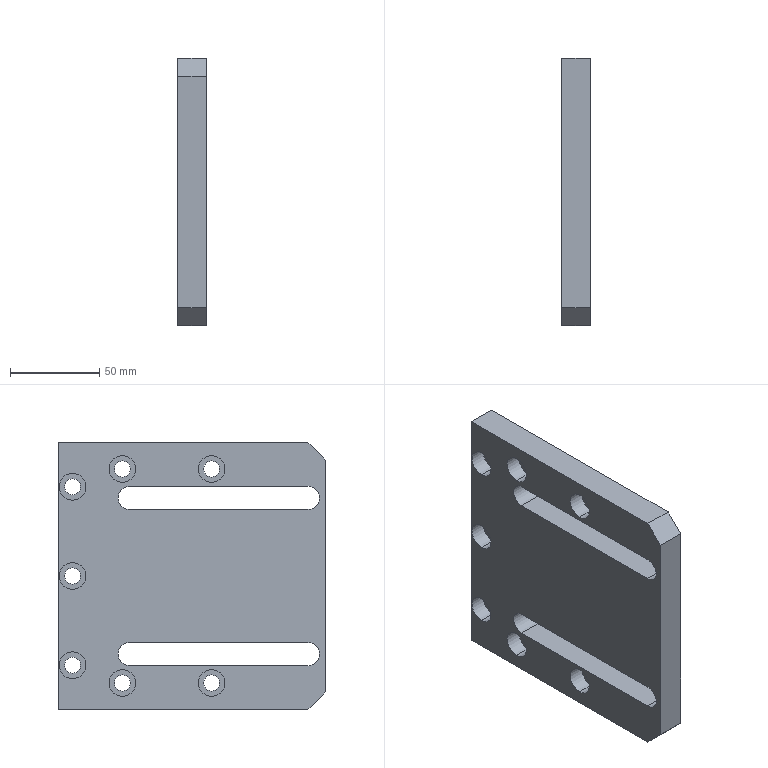Part | SolidWorks | features HoleWzd 2, Chamfer 1, Extrusion 1, ICE 1 | 1 solid | 51 faces | box 16 x 150 x 150 mm | volume 298302 mm3 | cylinder 32 | plane 19 | commonest cylinder face diameters 9 x14 15 x14 13 x4
STEP:
#1=CARTESIAN_POINT('',(9.,39.,-67.5));
#2=VERTEX_POINT('',#1);
#3=CARTESIAN_POINT('',(9.,39.,-52.5));
#4=VERTEX_POINT('',#3);
#5=CARTESIAN_POINT('',(9.,39.,-60.));
#6=DIRECTION('',(-1.,0.,0.));
#7=DIRECTION('',(0.,0.,1.));
#8=AXIS2_PLACEMENT_3D('',#5,#6,#7);
#9=CIRCLE('',#8,7.5);
#10=EDGE_CURVE('',#2,#4,#9,.T.);
#11=ORIENTED_EDGE('',*,*,#10,.F.);
#12=CARTESIAN_POINT('',(0.,39.,-67.5));
#13=VERTEX_POINT('',#12);
#14=CARTESIAN_POINT('',(0.,39.,-67.5));
#15=DIRECTION('',(-1.,0.,0.));
#16=VECTOR('',#15,1000.);
#17=LINE('',#14,#16);
#18=EDGE_CURVE('',#2,#13,#17,.T.);
#19=ORIENTED_EDGE('',*,*,#18,.T.);
#20=CARTESIAN_POINT('',(0.,39.,-52.5));
#21=VERTEX_POINT('',#20);
#22=CARTESIAN_POINT('',(0.,39.,-60.));
#23=DIRECTION('',(-1.,0.,0.));
#24=DIRECTION('',(0.,0.,1.));
#25=AXIS2_PLACEMENT_3D('',#22,#23,#24);
#26=CIRCLE('',#25,7.5);
#27=EDGE_CURVE('',#13,#21,#26,.T.);
#28=ORIENTED_EDGE('',*,*,#27,.T.);
#29=CARTESIAN_POINT('',(0.,39.,-52.5));
#30=DIRECTION('',(-1.,0.,0.));
#31=VECTOR('',#30,1000.);
#32=LINE('',#29,#31);
#33=EDGE_CURVE('',#4,#21,#32,.T.);
#34=ORIENTED_EDGE('',*,*,#33,.F.);
#35=EDGE_LOOP('',(#11,#19,#28,#34));
#36=FACE_OUTER_BOUND('',#35,.T.);
#37=CARTESIAN_POINT('',(0.,39.,-60.));
#38=DIRECTION('',(-1.,0.,0.));
#39=DIRECTION('',(0.,0.,1.));
#40=AXIS2_PLACEMENT_3D('',#37,#38,#39);
#41=CYLINDRICAL_SURFACE('',#40,7.5);
#42=ADVANCED_FACE('',(#36),#41,.F.);
#43=CARTESIAN_POINT('',(16.,39.,-55.5));
#44=VERTEX_POINT('',#43);
#45=CARTESIAN_POINT('',(16.,39.,-64.5));
#46=VERTEX_POINT('',#45);
#47=CARTESIAN_POINT('',(16.,39.,-60.));
#48=DIRECTION('',(1.,0.,0.));
#49=DIRECTION('',(0.,0.,-1.));
#50=AXIS2_PLACEMENT_3D('',#47,#48,#49);
#51=CIRCLE('',#50,4.5);
#52=EDGE_CURVE('',#44,#46,#51,.T.);
#53=ORIENTED_EDGE('',*,*,#52,.T.);
#54=CARTESIAN_POINT('',(9.,39.,-64.5));
#55=VERTEX_POINT('',#54);
#56=CARTESIAN_POINT('',(0.,39.,-64.5));
#57=DIRECTION('',(-1.,0.,0.));
#58=VECTOR('',#57,1000.);
#59=LINE('',#56,#58);
#60=EDGE_CURVE('',#46,#55,#59,.T.);
#61=ORIENTED_EDGE('',*,*,#60,.T.);
#62=CARTESIAN_POINT('',(9.,39.,-55.5));
#63=VERTEX_POINT('',#62);
#64=CARTESIAN_POINT('',(9.,39.,-60.));
#65=DIRECTION('',(-1.,0.,0.));
#66=DIRECTION('',(0.,0.,1.));
#67=AXIS2_PLACEMENT_3D('',#64,#65,#66);
#68=CIRCLE('',#67,4.5);
#69=EDGE_CURVE('',#55,#63,#68,.T.);
#70=ORIENTED_EDGE('',*,*,#69,.T.);
#71=CARTESIAN_POINT('',(0.,39.,-55.5));
#72=DIRECTION('',(-1.,0.,0.));
#73=VECTOR('',#72,1000.);
#74=LINE('',#71,#73);
#75=EDGE_CURVE('',#44,#63,#74,.T.);
#76=ORIENTED_EDGE('',*,*,#75,.F.);
#77=EDGE_LOOP('',(#53,#61,#70,#76));
#78=FACE_OUTER_BOUND('',#77,.T.);
#79=CARTESIAN_POINT('',(0.,39.,-60.));
#80=DIRECTION('',(-1.,0.,0.));
#81=DIRECTION('',(0.,0.,1.));
#82=AXIS2_PLACEMENT_3D('',#79,#80,#81);
#83=CYLINDRICAL_SURFACE('',#82,4.5);
#84=ADVANCED_FACE('',(#78),#83,.F.);
#85=CARTESIAN_POINT('',(9.,-11.,-67.5));
#86=VERTEX_POINT('',#85);
#87=CARTESIAN_POINT('',(9.,-11.,-52.5));
#88=VERTEX_POINT('',#87);
#89=CARTESIAN_POINT('',(9.,-11.,-60.));
#90=DIRECTION('',(-1.,0.,0.));
#91=DIRECTION('',(0.,0.,1.));
#92=AXIS2_PLACEMENT_3D('',#89,#90,#91);
#93=CIRCLE('',#92,7.5);
#94=EDGE_CURVE('',#86,#88,#93,.T.);
#95=ORIENTED_EDGE('',*,*,#94,.F.);
#96=CARTESIAN_POINT('',(0.,-11.,-67.5));
#97=VERTEX_POINT('',#96);
#98=CARTESIAN_POINT('',(0.,-11.,-67.5));
#99=DIRECTION('',(-1.,0.,0.));
#100=VECTOR('',#99,1000.);
#101=LINE('',#98,#100);
#102=EDGE_CURVE('',#86,#97,#101,.T.);
#103=ORIENTED_EDGE('',*,*,#102,.T.);
#104=CARTESIAN_POINT('',(0.,-11.,-52.5));
#105=VERTEX_POINT('',#104);
#106=CARTESIAN_POINT('',(0.,-11.,-60.));
#107=DIRECTION('',(-1.,0.,0.));
#108=DIRECTION('',(0.,0.,1.));
#109=AXIS2_PLACEMENT_3D('',#106,#107,#108);
#110=CIRCLE('',#109,7.5);
#111=EDGE_CURVE('',#97,#105,#110,.T.);
#112=ORIENTED_EDGE('',*,*,#111,.T.);
#113=CARTESIAN_POINT('',(0.,-11.,-52.5));
#114=DIRECTION('',(-1.,0.,0.));
#115=VECTOR('',#114,1000.);
#116=LINE('',#113,#115);
#117=EDGE_CURVE('',#88,#105,#116,.T.);
#118=ORIENTED_EDGE('',*,*,#117,.F.);
#119=EDGE_LOOP('',(#95,#103,#112,#118));
#120=FACE_OUTER_BOUND('',#119,.T.);
#121=CARTESIAN_POINT('',(0.,-11.,-60.));
#122=DIRECTION('',(-1.,0.,0.));
#123=DIRECTION('',(0.,0.,1.));
#124=AXIS2_PLACEMENT_3D('',#121,#122,#123);
#125=CYLINDRICAL_SURFACE('',#124,7.5);
#126=ADVANCED_FACE('',(#120),#125,.F.);
#127=CARTESIAN_POINT('',(16.,-11.,-55.5));
#128=VERTEX_POINT('',#127);
#129=CARTESIAN_POINT('',(16.,-11.,-64.5));
#130=VERTEX_POINT('',#129);
#131=CARTESIAN_POINT('',(16.,-11.,-60.));
#132=DIRECTION('',(1.,0.,0.));
#133=DIRECTION('',(0.,0.,-1.));
#134=AXIS2_PLACEMENT_3D('',#131,#132,#133);
#135=CIRCLE('',#134,4.5);
#136=EDGE_CURVE('',#128,#130,#135,.T.);
#137=ORIENTED_EDGE('',*,*,#136,.T.);
#138=CARTESIAN_POINT('',(9.,-11.,-64.5));
#139=VERTEX_POINT('',#138);
#140=CARTESIAN_POINT('',(0.,-11.,-64.5));
#141=DIRECTION('',(-1.,0.,0.));
#142=VECTOR('',#141,1000.);
#143=LINE('',#140,#142);
#144=EDGE_CURVE('',#130,#139,#143,.T.);
#145=ORIENTED_EDGE('',*,*,#144,.T.);
#146=CARTESIAN_POINT('',(9.,-11.,-55.5));
#147=VERTEX_POINT('',#146);
#148=CARTESIAN_POINT('',(9.,-11.,-60.));
#149=DIRECTION('',(-1.,0.,0.));
#150=DIRECTION('',(0.,0.,1.));
#151=AXIS2_PLACEMENT_3D('',#148,#149,#150);
#152=CIRCLE('',#151,4.5);
#153=EDGE_CURVE('',#139,#147,#152,.T.);
#154=ORIENTED_EDGE('',*,*,#153,.T.);
#155=CARTESIAN_POINT('',(0.,-11.,-55.5));
#156=DIRECTION('',(-1.,0.,0.));
#157=VECTOR('',#156,1000.);
#158=LINE('',#155,#157);
#159=EDGE_CURVE('',#128,#147,#158,.T.);
#160=ORIENTED_EDGE('',*,*,#159,.F.);
#161=EDGE_LOOP('',(#137,#145,#154,#160));
#162=FACE_OUTER_BOUND('',#161,.T.);
#163=CARTESIAN_POINT('',(0.,-11.,-60.));
#164=DIRECTION('',(-1.,0.,0.));
#165=DIRECTION('',(0.,0.,1.));
#166=AXIS2_PLACEMENT_3D('',#163,#164,#165);
#167=CYLINDRICAL_SURFACE('',#166,4.5);
#168=ADVANCED_FACE('',(#162),#167,.F.);
#169=CARTESIAN_POINT('',(9.,39.,52.5));
#170=VERTEX_POINT('',#169);
#171=CARTESIAN_POINT('',(9.,39.,67.5));
#172=VERTEX_POINT('',#171);
#173=CARTESIAN_POINT('',(9.,39.,60.));
#174=DIRECTION('',(-1.,0.,0.));
#175=DIRECTION('',(0.,0.,1.));
#176=AXIS2_PLACEMENT_3D('',#173,#174,#175);
#177=CIRCLE('',#176,7.5);
#178=EDGE_CURVE('',#170,#172,#177,.T.);
#179=ORIENTED_EDGE('',*,*,#178,.F.);
#180=CARTESIAN_POINT('',(0.,39.,52.5));
#181=VERTEX_POINT('',#180);
#182=CARTESIAN_POINT('',(0.,39.,52.5));
#183=DIRECTION('',(-1.,0.,0.));
#184=VECTOR('',#183,1000.);
#185=LINE('',#182,#184);
#186=EDGE_CURVE('',#170,#181,#185,.T.);
#187=ORIENTED_EDGE('',*,*,#186,.T.);
#188=CARTESIAN_POINT('',(0.,39.,67.5));
#189=VERTEX_POINT('',#188);
#190=CARTESIAN_POINT('',(0.,39.,60.));
#191=DIRECTION('',(-1.,0.,0.));
#192=DIRECTION('',(0.,0.,1.));
#193=AXIS2_PLACEMENT_3D('',#190,#191,#192);
#194=CIRCLE('',#193,7.5);
#195=EDGE_CURVE('',#181,#189,#194,.T.);
#196=ORIENTED_EDGE('',*,*,#195,.T.);
#197=CARTESIAN_POINT('',(0.,39.,67.5));
#198=DIRECTION('',(-1.,0.,0.));
#199=VECTOR('',#198,1000.);
#200=LINE('',#197,#199);
#201=EDGE_CURVE('',#172,#189,#200,.T.);
#202=ORIENTED_EDGE('',*,*,#201,.F.);
#203=EDGE_LOOP('',(#179,#187,#196,#202));
#204=FACE_OUTER_BOUND('',#203,.T.);
#205=CARTESIAN_POINT('',(0.,39.,60.));
#206=DIRECTION('',(-1.,0.,0.));
#207=DIRECTION('',(0.,0.,1.));
#208=AXIS2_PLACEMENT_3D('',#205,#206,#207);
#209=CYLINDRICAL_SURFACE('',#208,7.5);
#210=ADVANCED_FACE('',(#204),#209,.F.);
#211=CARTESIAN_POINT('',(16.,39.,64.5));
#212=VERTEX_POINT('',#211);
#213=CARTESIAN_POINT('',(16.,39.,55.5));
#214=VERTEX_POINT('',#213);
#215=CARTESIAN_POINT('',(16.,39.,60.));
#216=DIRECTION('',(1.,0.,0.));
#217=DIRECTION('',(0.,0.,-1.));
#218=AXIS2_PLACEMENT_3D('',#215,#216,#217);
#219=CIRCLE('',#218,4.5);
#220=EDGE_CURVE('',#212,#214,#219,.T.);
#221=ORIENTED_EDGE('',*,*,#220,.T.);
#222=CARTESIAN_POINT('',(9.,39.,55.5));
#223=VERTEX_POINT('',#222);
#224=CARTESIAN_POINT('',(0.,39.,55.5));
#225=DIRECTION('',(-1.,0.,0.));
#226=VECTOR('',#225,1000.);
#227=LINE('',#224,#226);
#228=EDGE_CURVE('',#214,#223,#227,.T.);
#229=ORIENTED_EDGE('',*,*,#228,.T.);
#230=CARTESIAN_POINT('',(9.,39.,64.5));
#231=VERTEX_POINT('',#230);
#232=CARTESIAN_POINT('',(9.,39.,60.));
#233=DIRECTION('',(-1.,0.,0.));
#234=DIRECTION('',(0.,0.,1.));
#235=AXIS2_PLACEMENT_3D('',#232,#233,#234);
#236=CIRCLE('',#235,4.5);
#237=EDGE_CURVE('',#223,#231,#236,.T.);
#238=ORIENTED_EDGE('',*,*,#237,.T.);
#239=CARTESIAN_POINT('',(0.,39.,64.5));
#240=DIRECTION('',(-1.,0.,0.));
#241=VECTOR('',#240,1000.);
#242=LINE('',#239,#241);
#243=EDGE_CURVE('',#212,#231,#242,.T.);
#244=ORIENTED_EDGE('',*,*,#243,.F.);
#245=EDGE_LOOP('',(#221,#229,#238,#244));
#246=FACE_OUTER_BOUND('',#245,.T.);
#247=CARTESIAN_POINT('',(0.,39.,60.));
#248=DIRECTION('',(-1.,0.,0.));
#249=DIRECTION('',(0.,0.,1.));
#250=AXIS2_PLACEMENT_3D('',#247,#248,#249);
#251=CYLINDRICAL_SURFACE('',#250,4.5);
#252=ADVANCED_FACE('',(#246),#251,.F.);
#253=CARTESIAN_POINT('',(9.,-11.,52.5));
#254=VERTEX_POINT('',#253);
#255=CARTESIAN_POINT('',(9.,-11.,67.5));
#256=VERTEX_POINT('',#255);
#257=CARTESIAN_POINT('',(9.,-11.,60.));
#258=DIRECTION('',(-1.,0.,0.));
#259=DIRECTION('',(0.,0.,1.));
#260=AXIS2_PLACEMENT_3D('',#257,#258,#259);
#261=CIRCLE('',#260,7.5);
#262=EDGE_CURVE('',#254,#256,#261,.T.);
#263=ORIENTED_EDGE('',*,*,#262,.F.);
#264=CARTESIAN_POINT('',(0.,-11.,52.5));
#265=VERTEX_POINT('',#264);
#266=CARTESIAN_POINT('',(0.,-11.,52.5));
#267=DIRECTION('',(-1.,0.,0.));
#268=VECTOR('',#267,1000.);
#269=LINE('',#266,#268);
#270=EDGE_CURVE('',#254,#265,#269,.T.);
#271=ORIENTED_EDGE('',*,*,#270,.T.);
#272=CARTESIAN_POINT('',(0.,-11.,67.5));
#273=VERTEX_POINT('',#272);
#274=CARTESIAN_POINT('',(0.,-11.,60.));
#275=DIRECTION('',(-1.,0.,0.));
#276=DIRECTION('',(0.,0.,1.));
#277=AXIS2_PLACEMENT_3D('',#274,#275,#276);
#278=CIRCLE('',#277,7.5);
#279=EDGE_CURVE('',#265,#273,#278,.T.);
#280=ORIENTED_EDGE('',*,*,#279,.T.);
#281=CARTESIAN_POINT('',(0.,-11.,67.5));
#282=DIRECTION('',(-1.,0.,0.));
#283=VECTOR('',#282,1000.);
#284=LINE('',#281,#283);
#285=EDGE_CURVE('',#256,#273,#284,.T.);
#286=ORIENTED_EDGE('',*,*,#285,.F.);
#287=EDGE_LOOP('',(#263,#271,#280,#286));
#288=FACE_OUTER_BOUND('',#287,.T.);
#289=CARTESIAN_POINT('',(0.,-11.,60.));
#290=DIRECTION('',(-1.,0.,0.));
#291=DIRECTION('',(0.,0.,1.));
#292=AXIS2_PLACEMENT_3D('',#289,#290,#291);
#293=CYLINDRICAL_SURFACE('',#292,7.5);
#294=ADVANCED_FACE('',(#288),#293,.F.);
#295=CARTESIAN_POINT('',(16.,-11.,64.5));
#296=VERTEX_POINT('',#295);
#297=CARTESIAN_POINT('',(16.,-11.,55.5));
#298=VERTEX_POINT('',#297);
#299=CARTESIAN_POINT('',(16.,-11.,60.));
#300=DIRECTION('',(1.,0.,0.));
#301=DIRECTION('',(0.,0.,-1.));
#302=AXIS2_PLACEMENT_3D('',#299,#300,#301);
#303=CIRCLE('',#302,4.5);
#304=EDGE_CURVE('',#296,#298,#303,.T.);
#305=ORIENTED_EDGE('',*,*,#304,.T.);
#306=CARTESIAN_POINT('',(9.,-11.,55.5));
#307=VERTEX_POINT('',#306);
#308=CARTESIAN_POINT('',(0.,-11.,55.5));
#309=DIRECTION('',(-1.,0.,0.));
#310=VECTOR('',#309,1000.);
#311=LINE('',#308,#310);
#312=EDGE_CURVE('',#298,#307,#311,.T.);
#313=ORIENTED_EDGE('',*,*,#312,.T.);
#314=CARTESIAN_POINT('',(9.,-11.,64.5));
#315=VERTEX_POINT('',#314);
#316=CARTESIAN_POINT('',(9.,-11.,60.));
#317=DIRECTION('',(-1.,0.,0.));
#318=DIRECTION('',(0.,0.,1.));
#319=AXIS2_PLACEMENT_3D('',#316,#317,#318);
#320=CIRCLE('',#319,4.5);
#321=EDGE_CURVE('',#307,#315,#320,.T.);
#322=ORIENTED_EDGE('',*,*,#321,.T.);
#323=CARTESIAN_POINT('',(0.,-11.,64.5));
#324=DIRECTION('',(-1.,0.,0.));
#325=VECTOR('',#324,1000.);
#326=LINE('',#323,#325);
#327=EDGE_CURVE('',#296,#315,#326,.T.);
#328=ORIENTED_EDGE('',*,*,#327,.F.);
#329=EDGE_LOOP('',(#305,#313,#322,#328));
#330=FACE_OUTER_BOUND('',#329,.T.);
#331=CARTESIAN_POINT('',(0.,-11.,60.));
#332=DIRECTION('',(-1.,0.,0.));
#333=DIRECTION('',(0.,0.,1.));
#334=AXIS2_PLACEMENT_3D('',#331,#332,#333);
#335=CYLINDRICAL_SURFACE('',#334,4.5);
#336=ADVANCED_FACE('',(#330),#335,.F.);
#337=CARTESIAN_POINT('',(9.,67.,-57.5));
#338=VERTEX_POINT('',#337);
#339=CARTESIAN_POINT('',(9.,67.,-42.5));
#340=VERTEX_POINT('',#339);
#341=CARTESIAN_POINT('',(9.,67.,-50.));
#342=DIRECTION('',(-1.,0.,0.));
#343=DIRECTION('',(0.,0.,1.));
#344=AXIS2_PLACEMENT_3D('',#341,#342,#343);
#345=CIRCLE('',#344,7.5);
#346=EDGE_CURVE('',#338,#340,#345,.T.);
#347=ORIENTED_EDGE('',*,*,#346,.F.);
#348=CARTESIAN_POINT('',(0.,67.,-57.5));
#349=VERTEX_POINT('',#348);
#350=CARTESIAN_POINT('',(0.,67.,-57.5));
#351=DIRECTION('',(-1.,0.,0.));
#352=VECTOR('',#351,1000.);
#353=LINE('',#350,#352);
#354=EDGE_CURVE('',#338,#349,#353,.T.);
#355=ORIENTED_EDGE('',*,*,#354,.T.);
#356=CARTESIAN_POINT('',(0.,67.,-42.5));
#357=VERTEX_POINT('',#356);
#358=CARTESIAN_POINT('',(0.,67.,-50.));
#359=DIRECTION('',(-1.,0.,0.));
#360=DIRECTION('',(0.,0.,1.));
#361=AXIS2_PLACEMENT_3D('',#358,#359,#360);
#362=CIRCLE('',#361,7.5);
#363=EDGE_CURVE('',#349,#357,#362,.T.);
#364=ORIENTED_EDGE('',*,*,#363,.T.);
#365=CARTESIAN_POINT('',(0.,67.,-42.5));
#366=DIRECTION('',(-1.,0.,0.));
#367=VECTOR('',#366,1000.);
#368=LINE('',#365,#367);
#369=EDGE_CURVE('',#340,#357,#368,.T.);
#370=ORIENTED_EDGE('',*,*,#369,.F.);
#371=EDGE_LOOP('',(#347,#355,#364,#370));
#372=FACE_OUTER_BOUND('',#371,.T.);
#373=CARTESIAN_POINT('',(0.,67.,-50.));
#374=DIRECTION('',(-1.,0.,0.));
#375=DIRECTION('',(0.,0.,1.));
#376=AXIS2_PLACEMENT_3D('',#373,#374,#375);
#377=CYLINDRICAL_SURFACE('',#376,7.5);
#378=ADVANCED_FACE('',(#372),#377,.F.);
#379=CARTESIAN_POINT('',(16.,67.,-45.5));
#380=VERTEX_POINT('',#379);
#381=CARTESIAN_POINT('',(16.,67.,-54.5));
#382=VERTEX_POINT('',#381);
#383=CARTESIAN_POINT('',(16.,67.,-50.));
#384=DIRECTION('',(1.,0.,0.));
#385=DIRECTION('',(0.,0.,-1.));
#386=AXIS2_PLACEMENT_3D('',#383,#384,#385);
#387=CIRCLE('',#386,4.5);
#388=EDGE_CURVE('',#380,#382,#387,.T.);
#389=ORIENTED_EDGE('',*,*,#388,.T.);
#390=CARTESIAN_POINT('',(9.,67.,-54.5));
#391=VERTEX_POINT('',#390);
#392=CARTESIAN_POINT('',(0.,67.,-54.5));
#393=DIRECTION('',(-1.,0.,0.));
#394=VECTOR('',#393,1000.);
#395=LINE('',#392,#394);
#396=EDGE_CURVE('',#382,#391,#395,.T.);
#397=ORIENTED_EDGE('',*,*,#396,.T.);
#398=CARTESIAN_POINT('',(9.,67.,-45.5));
#399=VERTEX_POINT('',#398);
#400=CARTESIAN_POINT('',(9.,67.,-50.));
#401=DIRECTION('',(-1.,0.,0.));
#402=DIRECTION('',(0.,0.,1.));
#403=AXIS2_PLACEMENT_3D('',#400,#401,#402);
#404=CIRCLE('',#403,4.5);
#405=EDGE_CURVE('',#391,#399,#404,.T.);
#406=ORIENTED_EDGE('',*,*,#405,.T.);
#407=CARTESIAN_POINT('',(0.,67.,-45.5));
#408=DIRECTION('',(-1.,0.,0.));
#409=VECTOR('',#408,1000.);
#410=LINE('',#407,#409);
#411=EDGE_CURVE('',#380,#399,#410,.T.);
#412=ORIENTED_EDGE('',*,*,#411,.F.);
#413=EDGE_LOOP('',(#389,#397,#406,#412));
#414=FACE_OUTER_BOUND('',#413,.T.);
#415=CARTESIAN_POINT('',(0.,67.,-50.));
#416=DIRECTION('',(-1.,0.,0.));
#417=DIRECTION('',(0.,0.,1.));
#418=AXIS2_PLACEMENT_3D('',#415,#416,#417);
#419=CYLINDRICAL_SURFACE('',#418,4.5);
#420=ADVANCED_FACE('',(#414),#419,.F.);
#421=CARTESIAN_POINT('',(9.,67.,-7.5));
#422=VERTEX_POINT('',#421);
#423=CARTESIAN_POINT('',(9.,67.,7.5));
#424=VERTEX_POINT('',#423);
#425=CARTESIAN_POINT('',(9.,67.,0.));
#426=DIRECTION('',(-1.,0.,0.));
#427=DIRECTION('',(0.,0.,1.));
#428=AXIS2_PLACEMENT_3D('',#425,#426,#427);
#429=CIRCLE('',#428,7.5);
#430=EDGE_CURVE('',#422,#424,#429,.T.);
#431=ORIENTED_EDGE('',*,*,#430,.F.);
#432=CARTESIAN_POINT('',(0.,67.,-7.5));
#433=VERTEX_POINT('',#432);
#434=CARTESIAN_POINT('',(0.,67.,-7.5));
#435=DIRECTION('',(-1.,0.,0.));
#436=VECTOR('',#435,1000.);
#437=LINE('',#434,#436);
#438=EDGE_CURVE('',#422,#433,#437,.T.);
#439=ORIENTED_EDGE('',*,*,#438,.T.);
#440=CARTESIAN_POINT('',(0.,67.,7.5));
#441=VERTEX_POINT('',#440);
#442=CARTESIAN_POINT('',(0.,67.,0.));
#443=DIRECTION('',(-1.,0.,0.));
#444=DIRECTION('',(0.,0.,1.));
#445=AXIS2_PLACEMENT_3D('',#442,#443,#444);
#446=CIRCLE('',#445,7.5);
#447=EDGE_CURVE('',#433,#441,#446,.T.);
#448=ORIENTED_EDGE('',*,*,#447,.T.);
#449=CARTESIAN_POINT('',(0.,67.,7.5));
#450=DIRECTION('',(-1.,0.,0.));
#451=VECTOR('',#450,1000.);
#452=LINE('',#449,#451);
#453=EDGE_CURVE('',#424,#441,#452,.T.);
#454=ORIENTED_EDGE('',*,*,#453,.F.);
#455=EDGE_LOOP('',(#431,#439,#448,#454));
#456=FACE_OUTER_BOUND('',#455,.T.);
#457=CARTESIAN_POINT('',(0.,67.,0.));
#458=DIRECTION('',(-1.,0.,0.));
#459=DIRECTION('',(0.,0.,1.));
#460=AXIS2_PLACEMENT_3D('',#457,#458,#459);
#461=CYLINDRICAL_SURFACE('',#460,7.5);
#462=ADVANCED_FACE('',(#456),#461,.F.);
#463=CARTESIAN_POINT('',(16.,67.,4.5));
#464=VERTEX_POINT('',#463);
#465=CARTESIAN_POINT('',(16.,67.,-4.5));
#466=VERTEX_POINT('',#465);
#467=CARTESIAN_POINT('',(16.,67.,0.));
#468=DIRECTION('',(1.,0.,0.));
#469=DIRECTION('',(0.,0.,-1.));
#470=AXIS2_PLACEMENT_3D('',#467,#468,#469);
#471=CIRCLE('',#470,4.5);
#472=EDGE_CURVE('',#464,#466,#471,.T.);
#473=ORIENTED_EDGE('',*,*,#472,.T.);
#474=CARTESIAN_POINT('',(9.,67.,-4.5));
#475=VERTEX_POINT('',#474);
#476=CARTESIAN_POINT('',(0.,67.,-4.5));
#477=DIRECTION('',(-1.,0.,0.));
#478=VECTOR('',#477,1000.);
#479=LINE('',#476,#478);
#480=EDGE_CURVE('',#466,#475,#479,.T.);
#481=ORIENTED_EDGE('',*,*,#480,.T.);
#482=CARTESIAN_POINT('',(9.,67.,4.5));
#483=VERTEX_POINT('',#482);
#484=CARTESIAN_POINT('',(9.,67.,0.));
#485=DIRECTION('',(-1.,0.,0.));
#486=DIRECTION('',(0.,0.,1.));
#487=AXIS2_PLACEMENT_3D('',#484,#485,#486);
#488=CIRCLE('',#487,4.5);
#489=EDGE_CURVE('',#475,#483,#488,.T.);
#490=ORIENTED_EDGE('',*,*,#489,.T.);
#491=CARTESIAN_POINT('',(0.,67.,4.5));
#492=DIRECTION('',(-1.,0.,0.));
#493=VECTOR('',#492,1000.);
#494=LINE('',#491,#493);
#495=EDGE_CURVE('',#464,#483,#494,.T.);
#496=ORIENTED_EDGE('',*,*,#495,.F.);
#497=EDGE_LOOP('',(#473,#481,#490,#496));
#498=FACE_OUTER_BOUND('',#497,.T.);
#499=CARTESIAN_POINT('',(0.,67.,0.));
#500=DIRECTION('',(-1.,0.,0.));
#501=DIRECTION('',(0.,0.,1.));
#502=AXIS2_PLACEMENT_3D('',#499,#500,#501);
#503=CYLINDRICAL_SURFACE('',#502,4.5);
#504=ADVANCED_FACE('',(#498),#503,.F.);
#505=CARTESIAN_POINT('',(9.,67.,42.5));
#506=VERTEX_POINT('',#505);
#507=CARTESIAN_POINT('',(9.,67.,57.5));
#508=VERTEX_POINT('',#507);
#509=CARTESIAN_POINT('',(9.,67.,50.));
#510=DIRECTION('',(-1.,0.,0.));
#511=DIRECTION('',(0.,0.,1.));
#512=AXIS2_PLACEMENT_3D('',#509,#510,#511);
#513=CIRCLE('',#512,7.5);
#514=EDGE_CURVE('',#506,#508,#513,.T.);
#515=ORIENTED_EDGE('',*,*,#514,.F.);
#516=CARTESIAN_POINT('',(0.,67.,42.5));
#517=VERTEX_POINT('',#516);
#518=CARTESIAN_POINT('',(0.,67.,42.5));
#519=DIRECTION('',(-1.,0.,0.));
#520=VECTOR('',#519,1000.);
#521=LINE('',#518,#520);
#522=EDGE_CURVE('',#506,#517,#521,.T.);
#523=ORIENTED_EDGE('',*,*,#522,.T.);
#524=CARTESIAN_POINT('',(0.,67.,57.5));
#525=VERTEX_POINT('',#524);
#526=CARTESIAN_POINT('',(0.,67.,50.));
#527=DIRECTION('',(-1.,0.,0.));
#528=DIRECTION('',(0.,0.,1.));
#529=AXIS2_PLACEMENT_3D('',#526,#527,#528);
#530=CIRCLE('',#529,7.5);
#531=EDGE_CURVE('',#517,#525,#530,.T.);
#532=ORIENTED_EDGE('',*,*,#531,.T.);
#533=CARTESIAN_POINT('',(0.,67.,57.5));
#534=DIRECTION('',(-1.,0.,0.));
#535=VECTOR('',#534,1000.);
#536=LINE('',#533,#535);
#537=EDGE_CURVE('',#508,#525,#536,.T.);
#538=ORIENTED_EDGE('',*,*,#537,.F.);
#539=EDGE_LOOP('',(#515,#523,#532,#538));
#540=FACE_OUTER_BOUND('',#539,.T.);
#541=CARTESIAN_POINT('',(0.,67.,50.));
#542=DIRECTION('',(-1.,0.,0.));
#543=DIRECTION('',(0.,0.,1.));
#544=AXIS2_PLACEMENT_3D('',#541,#542,#543);
#545=CYLINDRICAL_SURFACE('',#544,7.5);
#546=ADVANCED_FACE('',(#540),#545,.F.);
#547=CARTESIAN_POINT('',(16.,67.,54.5));
#548=VERTEX_POINT('',#547);
#549=CARTESIAN_POINT('',(16.,67.,45.5));
#550=VERTEX_POINT('',#549);
#551=CARTESIAN_POINT('',(16.,67.,50.));
#552=DIRECTION('',(1.,0.,0.));
#553=DIRECTION('',(0.,0.,-1.));
#554=AXIS2_PLACEMENT_3D('',#551,#552,#553);
#555=CIRCLE('',#554,4.5);
#556=EDGE_CURVE('',#548,#550,#555,.T.);
#557=ORIENTED_EDGE('',*,*,#556,.T.);
#558=CARTESIAN_POINT('',(9.,67.,45.5));
#559=VERTEX_POINT('',#558);
#560=CARTESIAN_POINT('',(0.,67.,45.5));
#561=DIRECTION('',(-1.,0.,0.));
#562=VECTOR('',#561,1000.);
#563=LINE('',#560,#562);
#564=EDGE_CURVE('',#550,#559,#563,.T.);
#565=ORIENTED_EDGE('',*,*,#564,.T.);
#566=CARTESIAN_POINT('',(9.,67.,54.5));
#567=VERTEX_POINT('',#566);
#568=CARTESIAN_POINT('',(9.,67.,50.));
#569=DIRECTION('',(-1.,0.,0.));
#570=DIRECTION('',(0.,0.,1.));
#571=AXIS2_PLACEMENT_3D('',#568,#569,#570);
#572=CIRCLE('',#571,4.5);
#573=EDGE_CURVE('',#559,#567,#572,.T.);
#574=ORIENTED_EDGE('',*,*,#573,.T.);
#575=CARTESIAN_POINT('',(0.,67.,54.5));
#576=DIRECTION('',(-1.,0.,0.));
#577=VECTOR('',#576,1000.);
#578=LINE('',#575,#577);
#579=EDGE_CURVE('',#548,#567,#578,.T.);
#580=ORIENTED_EDGE('',*,*,#579,.F.);
#581=EDGE_LOOP('',(#557,#565,#574,#580));
#582=FACE_OUTER_BOUND('',#581,.T.);
#583=CARTESIAN_POINT('',(0.,67.,50.));
#584=DIRECTION('',(-1.,0.,0.));
#585=DIRECTION('',(0.,0.,1.));
#586=AXIS2_PLACEMENT_3D('',#583,#584,#585);
#587=CYLINDRICAL_SURFACE('',#586,4.5);
#588=ADVANCED_FACE('',(#582),#587,.F.);
#589=CARTESIAN_POINT('',(16.,-65.,-75.));
#590=VERTEX_POINT('',#589);
#591=CARTESIAN_POINT('',(16.,75.,-75.));
#592=VERTEX_POINT('',#591);
#593=CARTESIAN_POINT('',(16.,75.,-75.));
#594=DIRECTION('',(0.,1.,0.));
#595=VECTOR('',#594,1000.);
#596=LINE('',#593,#595);
#597=EDGE_CURVE('',#590,#592,#596,.T.);
#598=ORIENTED_EDGE('',*,*,#597,.F.);
#599=CARTESIAN_POINT('',(0.,-65.,-75.));
#600=VERTEX_POINT('',#599);
#601=CARTESIAN_POINT('',(16.,-65.,-75.));
#602=DIRECTION('',(-1.,0.,0.));
#603=VECTOR('',#602,1000.);
#604=LINE('',#601,#603);
#605=EDGE_CURVE('',#590,#600,#604,.T.);
#606=ORIENTED_EDGE('',*,*,#605,.T.);
#607=CARTESIAN_POINT('',(0.,75.,-75.));
#608=VERTEX_POINT('',#607);
#609=CARTESIAN_POINT('',(0.,75.,-75.));
#610=DIRECTION('',(0.,1.,0.));
#611=VECTOR('',#610,1000.);
#612=LINE('',#609,#611);
#613=EDGE_CURVE('',#600,#608,#612,.T.);
#614=ORIENTED_EDGE('',*,*,#613,.T.);
#615=CARTESIAN_POINT('',(16.,75.,-75.));
#616=DIRECTION('',(-1.,0.,0.));
#617=VECTOR('',#616,1000.);
#618=LINE('',#615,#617);
#619=EDGE_CURVE('',#592,#608,#618,.T.);
#620=ORIENTED_EDGE('',*,*,#619,.F.);
#621=EDGE_LOOP('',(#598,#606,#614,#620));
#622=FACE_OUTER_BOUND('',#621,.T.);
#623=CARTESIAN_POINT('',(16.,75.,-75.));
#624=DIRECTION('',(0.,0.,1.));
#625=DIRECTION('',(0.,-1.,0.));
#626=AXIS2_PLACEMENT_3D('',#623,#624,#625);
#627=PLANE('',#626);
#628=ADVANCED_FACE('',(#622),#627,.F.);
#629=CARTESIAN_POINT('',(0.,75.,75.));
#630=VERTEX_POINT('',#629);
#631=CARTESIAN_POINT('',(0.,75.,75.));
#632=DIRECTION('',(0.,0.,1.));
#633=VECTOR('',#632,1000.);
#634=LINE('',#631,#633);
#635=EDGE_CURVE('',#608,#630,#634,.T.);
#636=ORIENTED_EDGE('',*,*,#635,.T.);
#637=CARTESIAN_POINT('',(16.,75.,75.));
#638=VERTEX_POINT('',#637);
#639=CARTESIAN_POINT('',(16.,75.,75.));
#640=DIRECTION('',(-1.,0.,0.));
#641=VECTOR('',#640,1000.);
#642=LINE('',#639,#641);
#643=EDGE_CURVE('',#638,#630,#642,.T.);
#644=ORIENTED_EDGE('',*,*,#643,.F.);
#645=CARTESIAN_POINT('',(16.,75.,75.));
#646=DIRECTION('',(0.,0.,1.));
#647=VECTOR('',#646,1000.);
#648=LINE('',#645,#647);
#649=EDGE_CURVE('',#592,#638,#648,.T.);
#650=ORIENTED_EDGE('',*,*,#649,.F.);
#651=ORIENTED_EDGE('',*,*,#619,.T.);
#652=EDGE_LOOP('',(#636,#644,#650,#651));
#653=FACE_OUTER_BOUND('',#652,.T.);
#654=CARTESIAN_POINT('',(16.,75.,75.));
#655=DIRECTION('',(0.,-1.,0.));
#656=DIRECTION('',(0.,0.,-1.));
#657=AXIS2_PLACEMENT_3D('',#654,#655,#656);
#658=PLANE('',#657);
#659=ADVANCED_FACE('',(#653),#658,.F.);
#660=CARTESIAN_POINT('',(0.,-65.,75.));
#661=VERTEX_POINT('',#660);
#662=CARTESIAN_POINT('',(0.,75.,75.));
#663=DIRECTION('',(0.,-1.,0.));
#664=VECTOR('',#663,1000.);
#665=LINE('',#662,#664);
#666=EDGE_CURVE('',#630,#661,#665,.T.);
#667=ORIENTED_EDGE('',*,*,#666,.T.);
#668=CARTESIAN_POINT('',(16.,-65.,75.));
#669=VERTEX_POINT('',#668);
#670=CARTESIAN_POINT('',(16.,-65.,75.));
#671=DIRECTION('',(1.,0.,0.));
#672=VECTOR('',#671,1000.);
#673=LINE('',#670,#672);
#674=EDGE_CURVE('',#661,#669,#673,.T.);
#675=ORIENTED_EDGE('',*,*,#674,.T.);
#676=CARTESIAN_POINT('',(16.,75.,75.));
#677=DIRECTION('',(0.,-1.,0.));
#678=VECTOR('',#677,1000.);
#679=LINE('',#676,#678);
#680=EDGE_CURVE('',#638,#669,#679,.T.);
#681=ORIENTED_EDGE('',*,*,#680,.F.);
#682=ORIENTED_EDGE('',*,*,#643,.T.);
#683=EDGE_LOOP('',(#667,#675,#681,#682));
#684=FACE_OUTER_BOUND('',#683,.T.);
#685=CARTESIAN_POINT('',(16.,75.,75.));
#686=DIRECTION('',(0.,0.,-1.));
#687=DIRECTION('',(0.,1.,0.));
#688=AXIS2_PLACEMENT_3D('',#685,#686,#687);
#689=PLANE('',#688);
#690=ADVANCED_FACE('',(#684),#689,.F.);
#691=CARTESIAN_POINT('',(16.,-75.,65.));
#692=VERTEX_POINT('',#691);
#693=CARTESIAN_POINT('',(16.,-75.,-65.));
#694=VERTEX_POINT('',#693);
#695=CARTESIAN_POINT('',(16.,-75.,75.));
#696=DIRECTION('',(0.,0.,-1.));
#697=VECTOR('',#696,1000.);
#698=LINE('',#695,#697);
#699=EDGE_CURVE('',#692,#694,#698,.T.);
#700=ORIENTED_EDGE('',*,*,#699,.F.);
#701=CARTESIAN_POINT('',(0.,-75.,65.));
#702=VERTEX_POINT('',#701);
#703=CARTESIAN_POINT('',(16.,-75.,65.));
#704=DIRECTION('',(-1.,0.,0.));
#705=VECTOR('',#704,1000.);
#706=LINE('',#703,#705);
#707=EDGE_CURVE('',#692,#702,#706,.T.);
#708=ORIENTED_EDGE('',*,*,#707,.T.);
#709=CARTESIAN_POINT('',(0.,-75.,-65.));
#710=VERTEX_POINT('',#709);
#711=CARTESIAN_POINT('',(0.,-75.,75.));
#712=DIRECTION('',(0.,0.,-1.));
#713=VECTOR('',#712,1000.);
#714=LINE('',#711,#713);
#715=EDGE_CURVE('',#702,#710,#714,.T.);
#716=ORIENTED_EDGE('',*,*,#715,.T.);
#717=CARTESIAN_POINT('',(16.,-75.,-65.));
#718=DIRECTION('',(1.,0.,0.));
#719=VECTOR('',#718,1000.);
#720=LINE('',#717,#719);
#721=EDGE_CURVE('',#710,#694,#720,.T.);
#722=ORIENTED_EDGE('',*,*,#721,.T.);
#723=EDGE_LOOP('',(#700,#708,#716,#722));
#724=FACE_OUTER_BOUND('',#723,.T.);
#725=CARTESIAN_POINT('',(16.,-75.,75.));
#726=DIRECTION('',(0.,1.,0.));
#727=DIRECTION('',(0.,0.,1.));
#728=AXIS2_PLACEMENT_3D('',#725,#726,#727);
#729=PLANE('',#728);
#730=ADVANCED_FACE('',(#724),#729,.F.);
#731=ORIENTED_EDGE('',*,*,#52,.F.);
#732=CARTESIAN_POINT('',(16.,39.,-60.));
#733=DIRECTION('',(1.,0.,0.));
#734=DIRECTION('',(0.,0.,-1.));
#735=AXIS2_PLACEMENT_3D('',#732,#733,#734);
#736=CIRCLE('',#735,4.5);
#737=EDGE_CURVE('',#46,#44,#736,.T.);
#738=ORIENTED_EDGE('',*,*,#737,.F.);
#739=EDGE_LOOP('',(#731,#738));
#740=FACE_BOUND('',#739,.T.);
#741=ORIENTED_EDGE('',*,*,#136,.F.);
#742=CARTESIAN_POINT('',(16.,-11.,-60.));
#743=DIRECTION('',(1.,0.,0.));
#744=DIRECTION('',(0.,0.,-1.));
#745=AXIS2_PLACEMENT_3D('',#742,#743,#744);
#746=CIRCLE('',#745,4.5);
#747=EDGE_CURVE('',#130,#128,#746,.T.);
#748=ORIENTED_EDGE('',*,*,#747,.F.);
#749=EDGE_LOOP('',(#741,#748));
#750=FACE_BOUND('',#749,.T.);
#751=ORIENTED_EDGE('',*,*,#220,.F.);
#752=CARTESIAN_POINT('',(16.,39.,60.));
#753=DIRECTION('',(1.,0.,0.));
#754=DIRECTION('',(0.,0.,-1.));
#755=AXIS2_PLACEMENT_3D('',#752,#753,#754);
#756=CIRCLE('',#755,4.5);
#757=EDGE_CURVE('',#214,#212,#756,.T.);
#758=ORIENTED_EDGE('',*,*,#757,.F.);
#759=EDGE_LOOP('',(#751,#758));
#760=FACE_BOUND('',#759,.T.);
#761=ORIENTED_EDGE('',*,*,#304,.F.);
#762=CARTESIAN_POINT('',(16.,-11.,60.));
#763=DIRECTION('',(1.,0.,0.));
#764=DIRECTION('',(0.,0.,-1.));
#765=AXIS2_PLACEMENT_3D('',#762,#763,#764);
#766=CIRCLE('',#765,4.5);
#767=EDGE_CURVE('',#298,#296,#766,.T.);
#768=ORIENTED_EDGE('',*,*,#767,.F.);
#769=EDGE_LOOP('',(#761,#768));
#770=FACE_BOUND('',#769,.T.);
#771=ORIENTED_EDGE('',*,*,#388,.F.);
#772=CARTESIAN_POINT('',(16.,67.,-50.));
#773=DIRECTION('',(1.,0.,0.));
#774=DIRECTION('',(0.,0.,-1.));
#775=AXIS2_PLACEMENT_3D('',#772,#773,#774);
#776=CIRCLE('',#775,4.5);
#777=EDGE_CURVE('',#382,#380,#776,.T.);
#778=ORIENTED_EDGE('',*,*,#777,.F.);
#779=EDGE_LOOP('',(#771,#778));
#780=FACE_BOUND('',#779,.T.);
#781=ORIENTED_EDGE('',*,*,#472,.F.);
#782=CARTESIAN_POINT('',(16.,67.,0.));
#783=DIRECTION('',(1.,0.,0.));
#784=DIRECTION('',(0.,0.,-1.));
#785=AXIS2_PLACEMENT_3D('',#782,#783,#784);
#786=CIRCLE('',#785,4.5);
#787=EDGE_CURVE('',#466,#464,#786,.T.);
#788=ORIENTED_EDGE('',*,*,#787,.F.);
#789=EDGE_LOOP('',(#781,#788));
#790=FACE_BOUND('',#789,.T.);
#791=ORIENTED_EDGE('',*,*,#556,.F.);
#792=CARTESIAN_POINT('',(16.,67.,50.));
#793=DIRECTION('',(1.,0.,0.));
#794=DIRECTION('',(0.,0.,-1.));
#795=AXIS2_PLACEMENT_3D('',#792,#793,#794);
#796=CIRCLE('',#795,4.5);
#797=EDGE_CURVE('',#550,#548,#796,.T.);
#798=ORIENTED_EDGE('',*,*,#797,.F.);
#799=EDGE_LOOP('',(#791,#798));
#800=FACE_BOUND('',#799,.T.);
#801=CARTESIAN_POINT('',(16.,35.,37.253));
#802=VERTEX_POINT('',#801);
#803=CARTESIAN_POINT('',(16.,35.,50.253));
#804=VERTEX_POINT('',#803);
#805=CARTESIAN_POINT('',(16.,35.,43.753));
#806=DIRECTION('',(1.,0.,0.));
#807=DIRECTION('',(0.,0.,-1.));
#808=AXIS2_PLACEMENT_3D('',#805,#806,#807);
#809=CIRCLE('',#808,6.5);
#810=EDGE_CURVE('',#802,#804,#809,.T.);
#811=ORIENTED_EDGE('',*,*,#810,.F.);
#812=CARTESIAN_POINT('',(16.,-65.,37.253));
#813=VERTEX_POINT('',#812);
#814=CARTESIAN_POINT('',(16.,35.,37.253));
#815=DIRECTION('',(0.,1.,0.));
#816=VECTOR('',#815,1000.);
#817=LINE('',#814,#816);
#818=EDGE_CURVE('',#813,#802,#817,.T.);
#819=ORIENTED_EDGE('',*,*,#818,.F.);
#820=CARTESIAN_POINT('',(16.,-65.,50.253));
#821=VERTEX_POINT('',#820);
#822=CARTESIAN_POINT('',(16.,-65.,43.753));
#823=DIRECTION('',(1.,0.,0.));
#824=DIRECTION('',(0.,0.,-1.));
#825=AXIS2_PLACEMENT_3D('',#822,#823,#824);
#826=CIRCLE('',#825,6.5);
#827=EDGE_CURVE('',#821,#813,#826,.T.);
#828=ORIENTED_EDGE('',*,*,#827,.F.);
#829=CARTESIAN_POINT('',(16.,35.,50.253));
#830=DIRECTION('',(0.,-1.,0.));
#831=VECTOR('',#830,1000.);
#832=LINE('',#829,#831);
#833=EDGE_CURVE('',#804,#821,#832,.T.);
#834=ORIENTED_EDGE('',*,*,#833,.F.);
#835=EDGE_LOOP('',(#811,#819,#828,#834));
#836=FACE_BOUND('',#835,.T.);
#837=CARTESIAN_POINT('',(16.,35.,-50.253));
#838=VERTEX_POINT('',#837);
#839=CARTESIAN_POINT('',(16.,35.,-37.253));
#840=VERTEX_POINT('',#839);
#841=CARTESIAN_POINT('',(16.,35.,-43.753));
#842=DIRECTION('',(1.,0.,0.));
#843=DIRECTION('',(0.,0.,-1.));
#844=AXIS2_PLACEMENT_3D('',#841,#842,#843);
#845=CIRCLE('',#844,6.5);
#846=EDGE_CURVE('',#838,#840,#845,.T.);
#847=ORIENTED_EDGE('',*,*,#846,.F.);
#848=CARTESIAN_POINT('',(16.,-65.,-50.253));
#849=VERTEX_POINT('',#848);
#850=CARTESIAN_POINT('',(16.,35.,-50.253));
#851=DIRECTION('',(0.,1.,0.));
#852=VECTOR('',#851,1000.);
#853=LINE('',#850,#852);
#854=EDGE_CURVE('',#849,#838,#853,.T.);
#855=ORIENTED_EDGE('',*,*,#854,.F.);
#856=CARTESIAN_POINT('',(16.,-65.,-37.253));
#857=VERTEX_POINT('',#856);
#858=CARTESIAN_POINT('',(16.,-65.,-43.753));
#859=DIRECTION('',(1.,0.,0.));
#860=DIRECTION('',(0.,0.,-1.));
#861=AXIS2_PLACEMENT_3D('',#858,#859,#860);
#862=CIRCLE('',#861,6.5);
#863=EDGE_CURVE('',#857,#849,#862,.T.);
#864=ORIENTED_EDGE('',*,*,#863,.F.);
#865=CARTESIAN_POINT('',(16.,35.,-37.253));
#866=DIRECTION('',(0.,-1.,0.));
#867=VECTOR('',#866,1000.);
#868=LINE('',#865,#867);
#869=EDGE_CURVE('',#840,#857,#868,.T.);
#870=ORIENTED_EDGE('',*,*,#869,.F.);
#871=EDGE_LOOP('',(#847,#855,#864,#870));
#872=FACE_BOUND('',#871,.T.);
#873=ORIENTED_EDGE('',*,*,#680,.T.);
#874=CARTESIAN_POINT('',(16.,-70.,70.));
#875=DIRECTION('',(0.,-0.7071,-0.7071));
#876=VECTOR('',#875,1000.);
#877=LINE('',#874,#876);
#878=EDGE_CURVE('',#669,#692,#877,.T.);
#879=ORIENTED_EDGE('',*,*,#878,.T.);
#880=ORIENTED_EDGE('',*,*,#699,.T.);
#881=CARTESIAN_POINT('',(16.,-70.,-70.));
#882=DIRECTION('',(0.,0.7071,-0.7071));
#883=VECTOR('',#882,1000.);
#884=LINE('',#881,#883);
#885=EDGE_CURVE('',#694,#590,#884,.T.);
#886=ORIENTED_EDGE('',*,*,#885,.T.);
#887=ORIENTED_EDGE('',*,*,#597,.T.);
#888=ORIENTED_EDGE('',*,*,#649,.T.);
#889=EDGE_LOOP('',(#873,#879,#880,#886,#887,#888));
#890=FACE_OUTER_BOUND('',#889,.T.);
#891=CARTESIAN_POINT('',(16.,0.,0.));
#892=DIRECTION('',(1.,0.,0.));
#893=DIRECTION('',(0.,0.,-1.));
#894=AXIS2_PLACEMENT_3D('',#891,#892,#893);
#895=PLANE('',#894);
#896=ADVANCED_FACE('',(#740,#750,#760,#770,#780,#790,#800,#836,#872,#890),#895,.T.);
#897=CARTESIAN_POINT('',(0.,39.,-60.));
#898=DIRECTION('',(-1.,0.,0.));
#899=DIRECTION('',(0.,0.,1.));
#900=AXIS2_PLACEMENT_3D('',#897,#898,#899);
#901=CIRCLE('',#900,7.5);
#902=EDGE_CURVE('',#21,#13,#901,.T.);
#903=ORIENTED_EDGE('',*,*,#902,.F.);
#904=ORIENTED_EDGE('',*,*,#27,.F.);
#905=EDGE_LOOP('',(#903,#904));
#906=FACE_BOUND('',#905,.T.);
#907=CARTESIAN_POINT('',(0.,-11.,-60.));
#908=DIRECTION('',(-1.,0.,0.));
#909=DIRECTION('',(0.,0.,1.));
#910=AXIS2_PLACEMENT_3D('',#907,#908,#909);
#911=CIRCLE('',#910,7.5);
#912=EDGE_CURVE('',#105,#97,#911,.T.);
#913=ORIENTED_EDGE('',*,*,#912,.F.);
#914=ORIENTED_EDGE('',*,*,#111,.F.);
#915=EDGE_LOOP('',(#913,#914));
#916=FACE_BOUND('',#915,.T.);
#917=CARTESIAN_POINT('',(0.,39.,60.));
#918=DIRECTION('',(-1.,0.,0.));
#919=DIRECTION('',(0.,0.,1.));
#920=AXIS2_PLACEMENT_3D('',#917,#918,#919);
#921=CIRCLE('',#920,7.5);
#922=EDGE_CURVE('',#189,#181,#921,.T.);
#923=ORIENTED_EDGE('',*,*,#922,.F.);
#924=ORIENTED_EDGE('',*,*,#195,.F.);
#925=EDGE_LOOP('',(#923,#924));
#926=FACE_BOUND('',#925,.T.);
#927=CARTESIAN_POINT('',(0.,-11.,60.));
#928=DIRECTION('',(-1.,0.,0.));
#929=DIRECTION('',(0.,0.,1.));
#930=AXIS2_PLACEMENT_3D('',#927,#928,#929);
#931=CIRCLE('',#930,7.5);
#932=EDGE_CURVE('',#273,#265,#931,.T.);
#933=ORIENTED_EDGE('',*,*,#932,.F.);
#934=ORIENTED_EDGE('',*,*,#279,.F.);
#935=EDGE_LOOP('',(#933,#934));
#936=FACE_BOUND('',#935,.T.);
#937=CARTESIAN_POINT('',(0.,67.,-50.));
#938=DIRECTION('',(-1.,0.,0.));
#939=DIRECTION('',(0.,0.,1.));
#940=AXIS2_PLACEMENT_3D('',#937,#938,#939);
#941=CIRCLE('',#940,7.5);
#942=EDGE_CURVE('',#357,#349,#941,.T.);
#943=ORIENTED_EDGE('',*,*,#942,.F.);
#944=ORIENTED_EDGE('',*,*,#363,.F.);
#945=EDGE_LOOP('',(#943,#944));
#946=FACE_BOUND('',#945,.T.);
#947=CARTESIAN_POINT('',(0.,67.,0.));
#948=DIRECTION('',(-1.,0.,0.));
#949=DIRECTION('',(0.,0.,1.));
#950=AXIS2_PLACEMENT_3D('',#947,#948,#949);
#951=CIRCLE('',#950,7.5);
#952=EDGE_CURVE('',#441,#433,#951,.T.);
#953=ORIENTED_EDGE('',*,*,#952,.F.);
#954=ORIENTED_EDGE('',*,*,#447,.F.);
#955=EDGE_LOOP('',(#953,#954));
#956=FACE_BOUND('',#955,.T.);
#957=CARTESIAN_POINT('',(0.,67.,50.));
#958=DIRECTION('',(-1.,0.,0.));
#959=DIRECTION('',(0.,0.,1.));
#960=AXIS2_PLACEMENT_3D('',#957,#958,#959);
#961=CIRCLE('',#960,7.5);
#962=EDGE_CURVE('',#525,#517,#961,.T.);
#963=ORIENTED_EDGE('',*,*,#962,.F.);
#964=ORIENTED_EDGE('',*,*,#531,.F.);
#965=EDGE_LOOP('',(#963,#964));
#966=FACE_BOUND('',#965,.T.);
#967=CARTESIAN_POINT('',(0.,-65.,37.253));
#968=VERTEX_POINT('',#967);
#969=CARTESIAN_POINT('',(0.,35.,37.253));
#970=VERTEX_POINT('',#969);
#971=CARTESIAN_POINT('',(0.,35.,37.253));
#972=DIRECTION('',(0.,1.,0.));
#973=VECTOR('',#972,1000.);
#974=LINE('',#971,#973);
#975=EDGE_CURVE('',#968,#970,#974,.T.);
#976=ORIENTED_EDGE('',*,*,#975,.T.);
#977=CARTESIAN_POINT('',(0.,35.,50.253));
#978=VERTEX_POINT('',#977);
#979=CARTESIAN_POINT('',(0.,35.,43.753));
#980=DIRECTION('',(1.,0.,0.));
#981=DIRECTION('',(0.,0.,-1.));
#982=AXIS2_PLACEMENT_3D('',#979,#980,#981);
#983=CIRCLE('',#982,6.5);
#984=EDGE_CURVE('',#970,#978,#983,.T.);
#985=ORIENTED_EDGE('',*,*,#984,.T.);
#986=CARTESIAN_POINT('',(0.,-65.,50.253));
#987=VERTEX_POINT('',#986);
#988=CARTESIAN_POINT('',(0.,35.,50.253));
#989=DIRECTION('',(0.,-1.,0.));
#990=VECTOR('',#989,1000.);
#991=LINE('',#988,#990);
#992=EDGE_CURVE('',#978,#987,#991,.T.);
#993=ORIENTED_EDGE('',*,*,#992,.T.);
#994=CARTESIAN_POINT('',(0.,-65.,43.753));
#995=DIRECTION('',(1.,0.,0.));
#996=DIRECTION('',(0.,0.,-1.));
#997=AXIS2_PLACEMENT_3D('',#994,#995,#996);
#998=CIRCLE('',#997,6.5);
#999=EDGE_CURVE('',#987,#968,#998,.T.);
#1000=ORIENTED_EDGE('',*,*,#999,.T.);
#1001=EDGE_LOOP('',(#976,#985,#993,#1000));
#1002=FACE_BOUND('',#1001,.T.);
#1003=CARTESIAN_POINT('',(0.,-65.,-50.253));
#1004=VERTEX_POINT('',#1003);
#1005=CARTESIAN_POINT('',(0.,35.,-50.253));
#1006=VERTEX_POINT('',#1005);
#1007=CARTESIAN_POINT('',(0.,35.,-50.253));
#1008=DIRECTION('',(0.,1.,0.));
#1009=VECTOR('',#1008,1000.);
#1010=LINE('',#1007,#1009);
#1011=EDGE_CURVE('',#1004,#1006,#1010,.T.);
#1012=ORIENTED_EDGE('',*,*,#1011,.T.);
#1013=CARTESIAN_POINT('',(0.,35.,-37.253));
#1014=VERTEX_POINT('',#1013);
#1015=CARTESIAN_POINT('',(0.,35.,-43.753));
#1016=DIRECTION('',(1.,0.,0.));
#1017=DIRECTION('',(0.,0.,-1.));
#1018=AXIS2_PLACEMENT_3D('',#1015,#1016,#1017);
#1019=CIRCLE('',#1018,6.5);
#1020=EDGE_CURVE('',#1006,#1014,#1019,.T.);
#1021=ORIENTED_EDGE('',*,*,#1020,.T.);
#1022=CARTESIAN_POINT('',(0.,-65.,-37.253));
#1023=VERTEX_POINT('',#1022);
#1024=CARTESIAN_POINT('',(0.,35.,-37.253));
#1025=DIRECTION('',(0.,-1.,0.));
#1026=VECTOR('',#1025,1000.);
#1027=LINE('',#1024,#1026);
#1028=EDGE_CURVE('',#1014,#1023,#1027,.T.);
#1029=ORIENTED_EDGE('',*,*,#1028,.T.);
#1030=CARTESIAN_POINT('',(0.,-65.,-43.753));
#1031=DIRECTION('',(1.,0.,0.));
#1032=DIRECTION('',(0.,0.,-1.));
#1033=AXIS2_PLACEMENT_3D('',#1030,#1031,#1032);
#1034=CIRCLE('',#1033,6.5);
#1035=EDGE_CURVE('',#1023,#1004,#1034,.T.);
#1036=ORIENTED_EDGE('',*,*,#1035,.T.);
#1037=EDGE_LOOP('',(#1012,#1021,#1029,#1036));
#1038=FACE_BOUND('',#1037,.T.);
#1039=ORIENTED_EDGE('',*,*,#715,.F.);
#1040=CARTESIAN_POINT('',(0.,-75.,65.));
#1041=DIRECTION('',(0.,0.7071,0.7071));
#1042=VECTOR('',#1041,1000.);
#1043=LINE('',#1040,#1042);
#1044=EDGE_CURVE('',#702,#661,#1043,.T.);
#1045=ORIENTED_EDGE('',*,*,#1044,.T.);
#1046=ORIENTED_EDGE('',*,*,#666,.F.);
#1047=ORIENTED_EDGE('',*,*,#635,.F.);
#1048=ORIENTED_EDGE('',*,*,#613,.F.);
#1049=CARTESIAN_POINT('',(0.,-65.,-75.));
#1050=DIRECTION('',(0.,-0.7071,0.7071));
#1051=VECTOR('',#1050,1000.);
#1052=LINE('',#1049,#1051);
#1053=EDGE_CURVE('',#600,#710,#1052,.T.);
#1054=ORIENTED_EDGE('',*,*,#1053,.T.);
#1055=EDGE_LOOP('',(#1039,#1045,#1046,#1047,#1048,#1054));
#1056=FACE_OUTER_BOUND('',#1055,.T.);
#1057=CARTESIAN_POINT('',(0.,0.,0.));
#1058=DIRECTION('',(1.,0.,0.));
#1059=DIRECTION('',(0.,0.,-1.));
#1060=AXIS2_PLACEMENT_3D('',#1057,#1058,#1059);
#1061=PLANE('',#1060);
#1062=ADVANCED_FACE('',(#906,#916,#926,#936,#946,#956,#966,#1002,#1038,#1056),#1061,.F.);
#1063=ORIENTED_EDGE('',*,*,#846,.T.);
#1064=CARTESIAN_POINT('',(0.,35.,-37.253));
#1065=DIRECTION('',(1.,0.,0.));
#1066=VECTOR('',#1065,1000.);
#1067=LINE('',#1064,#1066);
#1068=EDGE_CURVE('',#1014,#840,#1067,.T.);
#1069=ORIENTED_EDGE('',*,*,#1068,.F.);
#1070=ORIENTED_EDGE('',*,*,#1020,.F.);
#1071=CARTESIAN_POINT('',(0.,35.,-50.253));
#1072=DIRECTION('',(1.,0.,0.));
#1073=VECTOR('',#1072,1000.);
#1074=LINE('',#1071,#1073);
#1075=EDGE_CURVE('',#1006,#838,#1074,.T.);
#1076=ORIENTED_EDGE('',*,*,#1075,.T.);
#1077=EDGE_LOOP('',(#1063,#1069,#1070,#1076));
#1078=FACE_OUTER_BOUND('',#1077,.T.);
#1079=CARTESIAN_POINT('',(0.,35.,-43.753));
#1080=DIRECTION('',(1.,0.,0.));
#1081=DIRECTION('',(0.,0.,-1.));
#1082=AXIS2_PLACEMENT_3D('',#1079,#1080,#1081);
#1083=CYLINDRICAL_SURFACE('',#1082,6.5);
#1084=ADVANCED_FACE('',(#1078),#1083,.F.);
#1085=ORIENTED_EDGE('',*,*,#854,.T.);
#1086=ORIENTED_EDGE('',*,*,#1075,.F.);
#1087=ORIENTED_EDGE('',*,*,#1011,.F.);
#1088=CARTESIAN_POINT('',(0.,-65.,-50.253));
#1089=DIRECTION('',(1.,0.,0.));
#1090=VECTOR('',#1089,1000.);
#1091=LINE('',#1088,#1090);
#1092=EDGE_CURVE('',#1004,#849,#1091,.T.);
#1093=ORIENTED_EDGE('',*,*,#1092,.T.);
#1094=EDGE_LOOP('',(#1085,#1086,#1087,#1093));
#1095=FACE_OUTER_BOUND('',#1094,.T.);
#1096=CARTESIAN_POINT('',(0.,35.,-50.253));
#1097=DIRECTION('',(0.,0.,-1.));
#1098=DIRECTION('',(0.,1.,0.));
#1099=AXIS2_PLACEMENT_3D('',#1096,#1097,#1098);
#1100=PLANE('',#1099);
#1101=ADVANCED_FACE('',(#1095),#1100,.F.);
#1102=ORIENTED_EDGE('',*,*,#863,.T.);
#1103=ORIENTED_EDGE('',*,*,#1092,.F.);
#1104=ORIENTED_EDGE('',*,*,#1035,.F.);
#1105=CARTESIAN_POINT('',(0.,-65.,-37.253));
#1106=DIRECTION('',(1.,0.,0.));
#1107=VECTOR('',#1106,1000.);
#1108=LINE('',#1105,#1107);
#1109=EDGE_CURVE('',#1023,#857,#1108,.T.);
#1110=ORIENTED_EDGE('',*,*,#1109,.T.);
#1111=EDGE_LOOP('',(#1102,#1103,#1104,#1110));
#1112=FACE_OUTER_BOUND('',#1111,.T.);
#1113=CARTESIAN_POINT('',(0.,-65.,-43.753));
#1114=DIRECTION('',(1.,0.,0.));
#1115=DIRECTION('',(0.,0.,-1.));
#1116=AXIS2_PLACEMENT_3D('',#1113,#1114,#1115);
#1117=CYLINDRICAL_SURFACE('',#1116,6.5);
#1118=ADVANCED_FACE('',(#1112),#1117,.F.);
#1119=ORIENTED_EDGE('',*,*,#869,.T.);
#1120=ORIENTED_EDGE('',*,*,#1109,.F.);
#1121=ORIENTED_EDGE('',*,*,#1028,.F.);
#1122=ORIENTED_EDGE('',*,*,#1068,.T.);
#1123=EDGE_LOOP('',(#1119,#1120,#1121,#1122));
#1124=FACE_OUTER_BOUND('',#1123,.T.);
#1125=CARTESIAN_POINT('',(0.,35.,-37.253));
#1126=DIRECTION('',(0.,0.,1.));
#1127=DIRECTION('',(1.,0.,0.));
#1128=AXIS2_PLACEMENT_3D('',#1125,#1126,#1127);
#1129=PLANE('',#1128);
#1130=ADVANCED_FACE('',(#1124),#1129,.F.);
#1131=ORIENTED_EDGE('',*,*,#810,.T.);
#1132=CARTESIAN_POINT('',(0.,35.,50.253));
#1133=DIRECTION('',(1.,0.,0.));
#1134=VECTOR('',#1133,1000.);
#1135=LINE('',#1132,#1134);
#1136=EDGE_CURVE('',#978,#804,#1135,.T.);
#1137=ORIENTED_EDGE('',*,*,#1136,.F.);
#1138=ORIENTED_EDGE('',*,*,#984,.F.);
#1139=CARTESIAN_POINT('',(0.,35.,37.253));
#1140=DIRECTION('',(1.,0.,0.));
#1141=VECTOR('',#1140,1000.);
#1142=LINE('',#1139,#1141);
#1143=EDGE_CURVE('',#970,#802,#1142,.T.);
#1144=ORIENTED_EDGE('',*,*,#1143,.T.);
#1145=EDGE_LOOP('',(#1131,#1137,#1138,#1144));
#1146=FACE_OUTER_BOUND('',#1145,.T.);
#1147=CARTESIAN_POINT('',(0.,35.,43.753));
#1148=DIRECTION('',(1.,0.,0.));
#1149=DIRECTION('',(0.,0.,-1.));
#1150=AXIS2_PLACEMENT_3D('',#1147,#1148,#1149);
#1151=CYLINDRICAL_SURFACE('',#1150,6.5);
#1152=ADVANCED_FACE('',(#1146),#1151,.F.);
#1153=ORIENTED_EDGE('',*,*,#818,.T.);
#1154=ORIENTED_EDGE('',*,*,#1143,.F.);
#1155=ORIENTED_EDGE('',*,*,#975,.F.);
#1156=CARTESIAN_POINT('',(0.,-65.,37.253));
#1157=DIRECTION('',(1.,0.,0.));
#1158=VECTOR('',#1157,1000.);
#1159=LINE('',#1156,#1158);
#1160=EDGE_CURVE('',#968,#813,#1159,.T.);
#1161=ORIENTED_EDGE('',*,*,#1160,.T.);
#1162=EDGE_LOOP('',(#1153,#1154,#1155,#1161));
#1163=FACE_OUTER_BOUND('',#1162,.T.);
#1164=CARTESIAN_POINT('',(0.,35.,37.253));
#1165=DIRECTION('',(0.,0.,-1.));
#1166=DIRECTION('',(0.,1.,0.));
#1167=AXIS2_PLACEMENT_3D('',#1164,#1165,#1166);
#1168=PLANE('',#1167);
#1169=ADVANCED_FACE('',(#1163),#1168,.F.);
#1170=ORIENTED_EDGE('',*,*,#827,.T.);
#1171=ORIENTED_EDGE('',*,*,#1160,.F.);
#1172=ORIENTED_EDGE('',*,*,#999,.F.);
#1173=CARTESIAN_POINT('',(0.,-65.,50.253));
#1174=DIRECTION('',(1.,0.,0.));
#1175=VECTOR('',#1174,1000.);
#1176=LINE('',#1173,#1175);
#1177=EDGE_CURVE('',#987,#821,#1176,.T.);
#1178=ORIENTED_EDGE('',*,*,#1177,.T.);
#1179=EDGE_LOOP('',(#1170,#1171,#1172,#1178));
#1180=FACE_OUTER_BOUND('',#1179,.T.);
#1181=CARTESIAN_POINT('',(0.,-65.,43.753));
#1182=DIRECTION('',(1.,0.,0.));
#1183=DIRECTION('',(0.,0.,-1.));
#1184=AXIS2_PLACEMENT_3D('',#1181,#1182,#1183);
#1185=CYLINDRICAL_SURFACE('',#1184,6.5);
#1186=ADVANCED_FACE('',(#1180),#1185,.F.);
#1187=ORIENTED_EDGE('',*,*,#833,.T.);
#1188=ORIENTED_EDGE('',*,*,#1177,.F.);
#1189=ORIENTED_EDGE('',*,*,#992,.F.);
#1190=ORIENTED_EDGE('',*,*,#1136,.T.);
#1191=EDGE_LOOP('',(#1187,#1188,#1189,#1190));
#1192=FACE_OUTER_BOUND('',#1191,.T.);
#1193=CARTESIAN_POINT('',(0.,35.,50.253));
#1194=DIRECTION('',(0.,0.,1.));
#1195=DIRECTION('',(0.,-1.,0.));
#1196=AXIS2_PLACEMENT_3D('',#1193,#1194,#1195);
#1197=PLANE('',#1196);
#1198=ADVANCED_FACE('',(#1192),#1197,.F.);
#1199=ORIENTED_EDGE('',*,*,#564,.F.);
#1200=ORIENTED_EDGE('',*,*,#797,.T.);
#1201=ORIENTED_EDGE('',*,*,#579,.T.);
#1202=CARTESIAN_POINT('',(9.,67.,50.));
#1203=DIRECTION('',(-1.,0.,0.));
#1204=DIRECTION('',(0.,0.,1.));
#1205=AXIS2_PLACEMENT_3D('',#1202,#1203,#1204);
#1206=CIRCLE('',#1205,4.5);
#1207=EDGE_CURVE('',#567,#559,#1206,.T.);
#1208=ORIENTED_EDGE('',*,*,#1207,.T.);
#1209=EDGE_LOOP('',(#1199,#1200,#1201,#1208));
#1210=FACE_OUTER_BOUND('',#1209,.T.);
#1211=CARTESIAN_POINT('',(0.,67.,50.));
#1212=DIRECTION('',(-1.,0.,0.));
#1213=DIRECTION('',(0.,0.,1.));
#1214=AXIS2_PLACEMENT_3D('',#1211,#1212,#1213);
#1215=CYLINDRICAL_SURFACE('',#1214,4.5);
#1216=ADVANCED_FACE('',(#1210),#1215,.F.);
#1217=ORIENTED_EDGE('',*,*,#1207,.F.);
#1218=ORIENTED_EDGE('',*,*,#573,.F.);
#1219=EDGE_LOOP('',(#1217,#1218));
#1220=FACE_BOUND('',#1219,.T.);
#1221=CARTESIAN_POINT('',(9.,67.,50.));
#1222=DIRECTION('',(-1.,0.,0.));
#1223=DIRECTION('',(0.,0.,1.));
#1224=AXIS2_PLACEMENT_3D('',#1221,#1222,#1223);
#1225=CIRCLE('',#1224,7.5);
#1226=EDGE_CURVE('',#508,#506,#1225,.T.);
#1227=ORIENTED_EDGE('',*,*,#1226,.T.);
#1228=ORIENTED_EDGE('',*,*,#514,.T.);
#1229=EDGE_LOOP('',(#1227,#1228));
#1230=FACE_OUTER_BOUND('',#1229,.T.);
#1231=CARTESIAN_POINT('',(9.,71.5,50.));
#1232=DIRECTION('',(1.,0.,0.));
#1233=DIRECTION('',(0.,0.,-1.));
#1234=AXIS2_PLACEMENT_3D('',#1231,#1232,#1233);
#1235=PLANE('',#1234);
#1236=ADVANCED_FACE('',(#1220,#1230),#1235,.F.);
#1237=ORIENTED_EDGE('',*,*,#522,.F.);
#1238=ORIENTED_EDGE('',*,*,#1226,.F.);
#1239=ORIENTED_EDGE('',*,*,#537,.T.);
#1240=ORIENTED_EDGE('',*,*,#962,.T.);
#1241=EDGE_LOOP('',(#1237,#1238,#1239,#1240));
#1242=FACE_OUTER_BOUND('',#1241,.T.);
#1243=CARTESIAN_POINT('',(0.,67.,50.));
#1244=DIRECTION('',(-1.,0.,0.));
#1245=DIRECTION('',(0.,0.,1.));
#1246=AXIS2_PLACEMENT_3D('',#1243,#1244,#1245);
#1247=CYLINDRICAL_SURFACE('',#1246,7.5);
#1248=ADVANCED_FACE('',(#1242),#1247,.F.);
#1249=ORIENTED_EDGE('',*,*,#480,.F.);
#1250=ORIENTED_EDGE('',*,*,#787,.T.);
#1251=ORIENTED_EDGE('',*,*,#495,.T.);
#1252=CARTESIAN_POINT('',(9.,67.,0.));
#1253=DIRECTION('',(-1.,0.,0.));
#1254=DIRECTION('',(0.,0.,1.));
#1255=AXIS2_PLACEMENT_3D('',#1252,#1253,#1254);
#1256=CIRCLE('',#1255,4.5);
#1257=EDGE_CURVE('',#483,#475,#1256,.T.);
#1258=ORIENTED_EDGE('',*,*,#1257,.T.);
#1259=EDGE_LOOP('',(#1249,#1250,#1251,#1258));
#1260=FACE_OUTER_BOUND('',#1259,.T.);
#1261=CARTESIAN_POINT('',(0.,67.,0.));
#1262=DIRECTION('',(-1.,0.,0.));
#1263=DIRECTION('',(0.,0.,1.));
#1264=AXIS2_PLACEMENT_3D('',#1261,#1262,#1263);
#1265=CYLINDRICAL_SURFACE('',#1264,4.5);
#1266=ADVANCED_FACE('',(#1260),#1265,.F.);
#1267=ORIENTED_EDGE('',*,*,#1257,.F.);
#1268=ORIENTED_EDGE('',*,*,#489,.F.);
#1269=EDGE_LOOP('',(#1267,#1268));
#1270=FACE_BOUND('',#1269,.T.);
#1271=CARTESIAN_POINT('',(9.,67.,0.));
#1272=DIRECTION('',(-1.,0.,0.));
#1273=DIRECTION('',(0.,0.,1.));
#1274=AXIS2_PLACEMENT_3D('',#1271,#1272,#1273);
#1275=CIRCLE('',#1274,7.5);
#1276=EDGE_CURVE('',#424,#422,#1275,.T.);
#1277=ORIENTED_EDGE('',*,*,#1276,.T.);
#1278=ORIENTED_EDGE('',*,*,#430,.T.);
#1279=EDGE_LOOP('',(#1277,#1278));
#1280=FACE_OUTER_BOUND('',#1279,.T.);
#1281=CARTESIAN_POINT('',(9.,71.5,0.));
#1282=DIRECTION('',(1.,0.,0.));
#1283=DIRECTION('',(0.,0.,-1.));
#1284=AXIS2_PLACEMENT_3D('',#1281,#1282,#1283);
#1285=PLANE('',#1284);
#1286=ADVANCED_FACE('',(#1270,#1280),#1285,.F.);
#1287=ORIENTED_EDGE('',*,*,#438,.F.);
#1288=ORIENTED_EDGE('',*,*,#1276,.F.);
#1289=ORIENTED_EDGE('',*,*,#453,.T.);
#1290=ORIENTED_EDGE('',*,*,#952,.T.);
#1291=EDGE_LOOP('',(#1287,#1288,#1289,#1290));
#1292=FACE_OUTER_BOUND('',#1291,.T.);
#1293=CARTESIAN_POINT('',(0.,67.,0.));
#1294=DIRECTION('',(-1.,0.,0.));
#1295=DIRECTION('',(0.,0.,1.));
#1296=AXIS2_PLACEMENT_3D('',#1293,#1294,#1295);
#1297=CYLINDRICAL_SURFACE('',#1296,7.5);
#1298=ADVANCED_FACE('',(#1292),#1297,.F.);
#1299=ORIENTED_EDGE('',*,*,#396,.F.);
#1300=ORIENTED_EDGE('',*,*,#777,.T.);
#1301=ORIENTED_EDGE('',*,*,#411,.T.);
#1302=CARTESIAN_POINT('',(9.,67.,-50.));
#1303=DIRECTION('',(-1.,0.,0.));
#1304=DIRECTION('',(0.,0.,1.));
#1305=AXIS2_PLACEMENT_3D('',#1302,#1303,#1304);
#1306=CIRCLE('',#1305,4.5);
#1307=EDGE_CURVE('',#399,#391,#1306,.T.);
#1308=ORIENTED_EDGE('',*,*,#1307,.T.);
#1309=EDGE_LOOP('',(#1299,#1300,#1301,#1308));
#1310=FACE_OUTER_BOUND('',#1309,.T.);
#1311=CARTESIAN_POINT('',(0.,67.,-50.));
#1312=DIRECTION('',(-1.,0.,0.));
#1313=DIRECTION('',(0.,0.,1.));
#1314=AXIS2_PLACEMENT_3D('',#1311,#1312,#1313);
#1315=CYLINDRICAL_SURFACE('',#1314,4.5);
#1316=ADVANCED_FACE('',(#1310),#1315,.F.);
#1317=ORIENTED_EDGE('',*,*,#1307,.F.);
#1318=ORIENTED_EDGE('',*,*,#405,.F.);
#1319=EDGE_LOOP('',(#1317,#1318));
#1320=FACE_BOUND('',#1319,.T.);
#1321=CARTESIAN_POINT('',(9.,67.,-50.));
#1322=DIRECTION('',(-1.,0.,0.));
#1323=DIRECTION('',(0.,0.,1.));
#1324=AXIS2_PLACEMENT_3D('',#1321,#1322,#1323);
#1325=CIRCLE('',#1324,7.5);
#1326=EDGE_CURVE('',#340,#338,#1325,.T.);
#1327=ORIENTED_EDGE('',*,*,#1326,.T.);
#1328=ORIENTED_EDGE('',*,*,#346,.T.);
#1329=EDGE_LOOP('',(#1327,#1328));
#1330=FACE_OUTER_BOUND('',#1329,.T.);
#1331=CARTESIAN_POINT('',(9.,71.5,-50.));
#1332=DIRECTION('',(1.,0.,0.));
#1333=DIRECTION('',(0.,0.,-1.));
#1334=AXIS2_PLACEMENT_3D('',#1331,#1332,#1333);
#1335=PLANE('',#1334);
#1336=ADVANCED_FACE('',(#1320,#1330),#1335,.F.);
#1337=ORIENTED_EDGE('',*,*,#354,.F.);
#1338=ORIENTED_EDGE('',*,*,#1326,.F.);
#1339=ORIENTED_EDGE('',*,*,#369,.T.);
#1340=ORIENTED_EDGE('',*,*,#942,.T.);
#1341=EDGE_LOOP('',(#1337,#1338,#1339,#1340));
#1342=FACE_OUTER_BOUND('',#1341,.T.);
#1343=CARTESIAN_POINT('',(0.,67.,-50.));
#1344=DIRECTION('',(-1.,0.,0.));
#1345=DIRECTION('',(0.,0.,1.));
#1346=AXIS2_PLACEMENT_3D('',#1343,#1344,#1345);
#1347=CYLINDRICAL_SURFACE('',#1346,7.5);
#1348=ADVANCED_FACE('',(#1342),#1347,.F.);
#1349=ORIENTED_EDGE('',*,*,#312,.F.);
#1350=ORIENTED_EDGE('',*,*,#767,.T.);
#1351=ORIENTED_EDGE('',*,*,#327,.T.);
#1352=CARTESIAN_POINT('',(9.,-11.,60.));
#1353=DIRECTION('',(-1.,0.,0.));
#1354=DIRECTION('',(0.,0.,1.));
#1355=AXIS2_PLACEMENT_3D('',#1352,#1353,#1354);
#1356=CIRCLE('',#1355,4.5);
#1357=EDGE_CURVE('',#315,#307,#1356,.T.);
#1358=ORIENTED_EDGE('',*,*,#1357,.T.);
#1359=EDGE_LOOP('',(#1349,#1350,#1351,#1358));
#1360=FACE_OUTER_BOUND('',#1359,.T.);
#1361=CARTESIAN_POINT('',(0.,-11.,60.));
#1362=DIRECTION('',(-1.,0.,0.));
#1363=DIRECTION('',(0.,0.,1.));
#1364=AXIS2_PLACEMENT_3D('',#1361,#1362,#1363);
#1365=CYLINDRICAL_SURFACE('',#1364,4.5);
#1366=ADVANCED_FACE('',(#1360),#1365,.F.);
#1367=ORIENTED_EDGE('',*,*,#1357,.F.);
#1368=ORIENTED_EDGE('',*,*,#321,.F.);
#1369=EDGE_LOOP('',(#1367,#1368));
#1370=FACE_BOUND('',#1369,.T.);
#1371=CARTESIAN_POINT('',(9.,-11.,60.));
#1372=DIRECTION('',(-1.,0.,0.));
#1373=DIRECTION('',(0.,0.,1.));
#1374=AXIS2_PLACEMENT_3D('',#1371,#1372,#1373);
#1375=CIRCLE('',#1374,7.5);
#1376=EDGE_CURVE('',#256,#254,#1375,.T.);
#1377=ORIENTED_EDGE('',*,*,#1376,.T.);
#1378=ORIENTED_EDGE('',*,*,#262,.T.);
#1379=EDGE_LOOP('',(#1377,#1378));
#1380=FACE_OUTER_BOUND('',#1379,.T.);
#1381=CARTESIAN_POINT('',(9.,-6.5,60.));
#1382=DIRECTION('',(1.,0.,0.));
#1383=DIRECTION('',(0.,0.,-1.));
#1384=AXIS2_PLACEMENT_3D('',#1381,#1382,#1383);
#1385=PLANE('',#1384);
#1386=ADVANCED_FACE('',(#1370,#1380),#1385,.F.);
#1387=ORIENTED_EDGE('',*,*,#270,.F.);
#1388=ORIENTED_EDGE('',*,*,#1376,.F.);
#1389=ORIENTED_EDGE('',*,*,#285,.T.);
#1390=ORIENTED_EDGE('',*,*,#932,.T.);
#1391=EDGE_LOOP('',(#1387,#1388,#1389,#1390));
#1392=FACE_OUTER_BOUND('',#1391,.T.);
#1393=CARTESIAN_POINT('',(0.,-11.,60.));
#1394=DIRECTION('',(-1.,0.,0.));
#1395=DIRECTION('',(0.,0.,1.));
#1396=AXIS2_PLACEMENT_3D('',#1393,#1394,#1395);
#1397=CYLINDRICAL_SURFACE('',#1396,7.5);
#1398=ADVANCED_FACE('',(#1392),#1397,.F.);
#1399=ORIENTED_EDGE('',*,*,#228,.F.);
#1400=ORIENTED_EDGE('',*,*,#757,.T.);
#1401=ORIENTED_EDGE('',*,*,#243,.T.);
#1402=CARTESIAN_POINT('',(9.,39.,60.));
#1403=DIRECTION('',(-1.,0.,0.));
#1404=DIRECTION('',(0.,0.,1.));
#1405=AXIS2_PLACEMENT_3D('',#1402,#1403,#1404);
#1406=CIRCLE('',#1405,4.5);
#1407=EDGE_CURVE('',#231,#223,#1406,.T.);
#1408=ORIENTED_EDGE('',*,*,#1407,.T.);
#1409=EDGE_LOOP('',(#1399,#1400,#1401,#1408));
#1410=FACE_OUTER_BOUND('',#1409,.T.);
#1411=CARTESIAN_POINT('',(0.,39.,60.));
#1412=DIRECTION('',(-1.,0.,0.));
#1413=DIRECTION('',(0.,0.,1.));
#1414=AXIS2_PLACEMENT_3D('',#1411,#1412,#1413);
#1415=CYLINDRICAL_SURFACE('',#1414,4.5);
#1416=ADVANCED_FACE('',(#1410),#1415,.F.);
#1417=ORIENTED_EDGE('',*,*,#1407,.F.);
#1418=ORIENTED_EDGE('',*,*,#237,.F.);
#1419=EDGE_LOOP('',(#1417,#1418));
#1420=FACE_BOUND('',#1419,.T.);
#1421=CARTESIAN_POINT('',(9.,39.,60.));
#1422=DIRECTION('',(-1.,0.,0.));
#1423=DIRECTION('',(0.,0.,1.));
#1424=AXIS2_PLACEMENT_3D('',#1421,#1422,#1423);
#1425=CIRCLE('',#1424,7.5);
#1426=EDGE_CURVE('',#172,#170,#1425,.T.);
#1427=ORIENTED_EDGE('',*,*,#1426,.T.);
#1428=ORIENTED_EDGE('',*,*,#178,.T.);
#1429=EDGE_LOOP('',(#1427,#1428));
#1430=FACE_OUTER_BOUND('',#1429,.T.);
#1431=CARTESIAN_POINT('',(9.,43.5,60.));
#1432=DIRECTION('',(1.,0.,0.));
#1433=DIRECTION('',(0.,0.,-1.));
#1434=AXIS2_PLACEMENT_3D('',#1431,#1432,#1433);
#1435=PLANE('',#1434);
#1436=ADVANCED_FACE('',(#1420,#1430),#1435,.F.);
#1437=ORIENTED_EDGE('',*,*,#186,.F.);
#1438=ORIENTED_EDGE('',*,*,#1426,.F.);
#1439=ORIENTED_EDGE('',*,*,#201,.T.);
#1440=ORIENTED_EDGE('',*,*,#922,.T.);
#1441=EDGE_LOOP('',(#1437,#1438,#1439,#1440));
#1442=FACE_OUTER_BOUND('',#1441,.T.);
#1443=CARTESIAN_POINT('',(0.,39.,60.));
#1444=DIRECTION('',(-1.,0.,0.));
#1445=DIRECTION('',(0.,0.,1.));
#1446=AXIS2_PLACEMENT_3D('',#1443,#1444,#1445);
#1447=CYLINDRICAL_SURFACE('',#1446,7.5);
#1448=ADVANCED_FACE('',(#1442),#1447,.F.);
#1449=ORIENTED_EDGE('',*,*,#144,.F.);
#1450=ORIENTED_EDGE('',*,*,#747,.T.);
#1451=ORIENTED_EDGE('',*,*,#159,.T.);
#1452=CARTESIAN_POINT('',(9.,-11.,-60.));
#1453=DIRECTION('',(-1.,0.,0.));
#1454=DIRECTION('',(0.,0.,1.));
#1455=AXIS2_PLACEMENT_3D('',#1452,#1453,#1454);
#1456=CIRCLE('',#1455,4.5);
#1457=EDGE_CURVE('',#147,#139,#1456,.T.);
#1458=ORIENTED_EDGE('',*,*,#1457,.T.);
#1459=EDGE_LOOP('',(#1449,#1450,#1451,#1458));
#1460=FACE_OUTER_BOUND('',#1459,.T.);
#1461=CARTESIAN_POINT('',(0.,-11.,-60.));
#1462=DIRECTION('',(-1.,0.,0.));
#1463=DIRECTION('',(0.,0.,1.));
#1464=AXIS2_PLACEMENT_3D('',#1461,#1462,#1463);
#1465=CYLINDRICAL_SURFACE('',#1464,4.5);
#1466=ADVANCED_FACE('',(#1460),#1465,.F.);
#1467=ORIENTED_EDGE('',*,*,#1457,.F.);
#1468=ORIENTED_EDGE('',*,*,#153,.F.);
#1469=EDGE_LOOP('',(#1467,#1468));
#1470=FACE_BOUND('',#1469,.T.);
#1471=CARTESIAN_POINT('',(9.,-11.,-60.));
#1472=DIRECTION('',(-1.,0.,0.));
#1473=DIRECTION('',(0.,0.,1.));
#1474=AXIS2_PLACEMENT_3D('',#1471,#1472,#1473);
#1475=CIRCLE('',#1474,7.5);
#1476=EDGE_CURVE('',#88,#86,#1475,.T.);
#1477=ORIENTED_EDGE('',*,*,#1476,.T.);
#1478=ORIENTED_EDGE('',*,*,#94,.T.);
#1479=EDGE_LOOP('',(#1477,#1478));
#1480=FACE_OUTER_BOUND('',#1479,.T.);
#1481=CARTESIAN_POINT('',(9.,-6.5,-60.));
#1482=DIRECTION('',(1.,0.,0.));
#1483=DIRECTION('',(0.,0.,-1.));
#1484=AXIS2_PLACEMENT_3D('',#1481,#1482,#1483);
#1485=PLANE('',#1484);
#1486=ADVANCED_FACE('',(#1470,#1480),#1485,.F.);
#1487=ORIENTED_EDGE('',*,*,#102,.F.);
#1488=ORIENTED_EDGE('',*,*,#1476,.F.);
#1489=ORIENTED_EDGE('',*,*,#117,.T.);
#1490=ORIENTED_EDGE('',*,*,#912,.T.);
#1491=EDGE_LOOP('',(#1487,#1488,#1489,#1490));
#1492=FACE_OUTER_BOUND('',#1491,.T.);
#1493=CARTESIAN_POINT('',(0.,-11.,-60.));
#1494=DIRECTION('',(-1.,0.,0.));
#1495=DIRECTION('',(0.,0.,1.));
#1496=AXIS2_PLACEMENT_3D('',#1493,#1494,#1495);
#1497=CYLINDRICAL_SURFACE('',#1496,7.5);
#1498=ADVANCED_FACE('',(#1492),#1497,.F.);
#1499=ORIENTED_EDGE('',*,*,#60,.F.);
#1500=ORIENTED_EDGE('',*,*,#737,.T.);
#1501=ORIENTED_EDGE('',*,*,#75,.T.);
#1502=CARTESIAN_POINT('',(9.,39.,-60.));
#1503=DIRECTION('',(-1.,0.,0.));
#1504=DIRECTION('',(0.,0.,1.));
#1505=AXIS2_PLACEMENT_3D('',#1502,#1503,#1504);
#1506=CIRCLE('',#1505,4.5);
#1507=EDGE_CURVE('',#63,#55,#1506,.T.);
#1508=ORIENTED_EDGE('',*,*,#1507,.T.);
#1509=EDGE_LOOP('',(#1499,#1500,#1501,#1508));
#1510=FACE_OUTER_BOUND('',#1509,.T.);
#1511=CARTESIAN_POINT('',(0.,39.,-60.));
#1512=DIRECTION('',(-1.,0.,0.));
#1513=DIRECTION('',(0.,0.,1.));
#1514=AXIS2_PLACEMENT_3D('',#1511,#1512,#1513);
#1515=CYLINDRICAL_SURFACE('',#1514,4.5);
#1516=ADVANCED_FACE('',(#1510),#1515,.F.);
#1517=ORIENTED_EDGE('',*,*,#1507,.F.);
#1518=ORIENTED_EDGE('',*,*,#69,.F.);
#1519=EDGE_LOOP('',(#1517,#1518));
#1520=FACE_BOUND('',#1519,.T.);
#1521=CARTESIAN_POINT('',(9.,39.,-60.));
#1522=DIRECTION('',(-1.,0.,0.));
#1523=DIRECTION('',(0.,0.,1.));
#1524=AXIS2_PLACEMENT_3D('',#1521,#1522,#1523);
#1525=CIRCLE('',#1524,7.5);
#1526=EDGE_CURVE('',#4,#2,#1525,.T.);
#1527=ORIENTED_EDGE('',*,*,#1526,.T.);
#1528=ORIENTED_EDGE('',*,*,#10,.T.);
#1529=EDGE_LOOP('',(#1527,#1528));
#1530=FACE_OUTER_BOUND('',#1529,.T.);
#1531=CARTESIAN_POINT('',(9.,43.5,-60.));
#1532=DIRECTION('',(1.,0.,0.));
#1533=DIRECTION('',(0.,0.,-1.));
#1534=AXIS2_PLACEMENT_3D('',#1531,#1532,#1533);
#1535=PLANE('',#1534);
#1536=ADVANCED_FACE('',(#1520,#1530),#1535,.F.);
#1537=ORIENTED_EDGE('',*,*,#18,.F.);
#1538=ORIENTED_EDGE('',*,*,#1526,.F.);
#1539=ORIENTED_EDGE('',*,*,#33,.T.);
#1540=ORIENTED_EDGE('',*,*,#902,.T.);
#1541=EDGE_LOOP('',(#1537,#1538,#1539,#1540));
#1542=FACE_OUTER_BOUND('',#1541,.T.);
#1543=CARTESIAN_POINT('',(0.,39.,-60.));
#1544=DIRECTION('',(-1.,0.,0.));
#1545=DIRECTION('',(0.,0.,1.));
#1546=AXIS2_PLACEMENT_3D('',#1543,#1544,#1545);
#1547=CYLINDRICAL_SURFACE('',#1546,7.5);
#1548=ADVANCED_FACE('',(#1542),#1547,.F.);
#1549=ORIENTED_EDGE('',*,*,#878,.F.);
#1550=ORIENTED_EDGE('',*,*,#674,.F.);
#1551=ORIENTED_EDGE('',*,*,#1044,.F.);
#1552=ORIENTED_EDGE('',*,*,#707,.F.);
#1553=EDGE_LOOP('',(#1549,#1550,#1551,#1552));
#1554=FACE_OUTER_BOUND('',#1553,.T.);
#1555=CARTESIAN_POINT('',(16.,-75.,65.));
#1556=DIRECTION('',(0.,0.7071,-0.7071));
#1557=DIRECTION('',(-1.,0.,0.));
#1558=AXIS2_PLACEMENT_3D('',#1555,#1556,#1557);
#1559=PLANE('',#1558);
#1560=ADVANCED_FACE('',(#1554),#1559,.F.);
#1561=ORIENTED_EDGE('',*,*,#885,.F.);
#1562=ORIENTED_EDGE('',*,*,#721,.F.);
#1563=ORIENTED_EDGE('',*,*,#1053,.F.);
#1564=ORIENTED_EDGE('',*,*,#605,.F.);
#1565=EDGE_LOOP('',(#1561,#1562,#1563,#1564));
#1566=FACE_OUTER_BOUND('',#1565,.T.);
#1567=CARTESIAN_POINT('',(16.,-65.,-75.));
#1568=DIRECTION('',(0.,0.7071,0.7071));
#1569=DIRECTION('',(-1.,0.,0.));
#1570=AXIS2_PLACEMENT_3D('',#1567,#1568,#1569);
#1571=PLANE('',#1570);
#1572=ADVANCED_FACE('',(#1566),#1571,.F.);
#1573=CLOSED_SHELL('',(#42,#84,#126,#168,#210,#252,#294,#336,#378,#420,#462,#504,#546,#588,#628,#659,#690,#730,#896,#1062,#1084,#1101,#1118,#1130,#1152,#1169,#1186,#1198,#1216,#1236,#1248,#1266,#1286,#1298,#1316,#1336,#1348,#1366,#1386,#1398,#1416,#1436,#1448,#1466,#1486,#1498,#1516,#1536,#1548,#1560,#1572));
#1574=MANIFOLD_SOLID_BREP('',#1573);
#1575=CARTESIAN_POINT('',(0.,0.,0.));
#1576=DIRECTION('',(0.,0.,1.));
#1577=DIRECTION('',(1.,0.,0.));
#1578=AXIS2_PLACEMENT_3D('',#1575,#1576,#1577);
#1579=(LENGTH_UNIT()NAMED_UNIT(*)SI_UNIT(.MILLI.,.METRE.));
#1580=UNCERTAINTY_MEASURE_WITH_UNIT(LENGTH_MEASURE(0.00001),#1579,'','');
#1581=(NAMED_UNIT(*)PLANE_ANGLE_UNIT()SI_UNIT($,.RADIAN.));
#1582=(NAMED_UNIT(*)SI_UNIT($,.STERADIAN.)SOLID_ANGLE_UNIT());
#1583=(GEOMETRIC_REPRESENTATION_CONTEXT(3)GLOBAL_UNCERTAINTY_ASSIGNED_CONTEXT((#1580))GLOBAL_UNIT_ASSIGNED_CONTEXT((#1579,#1581,#1582))REPRESENTATION_CONTEXT('',''));
#1584=ADVANCED_BREP_SHAPE_REPRESENTATION('',(#1574,#1578),#1583);